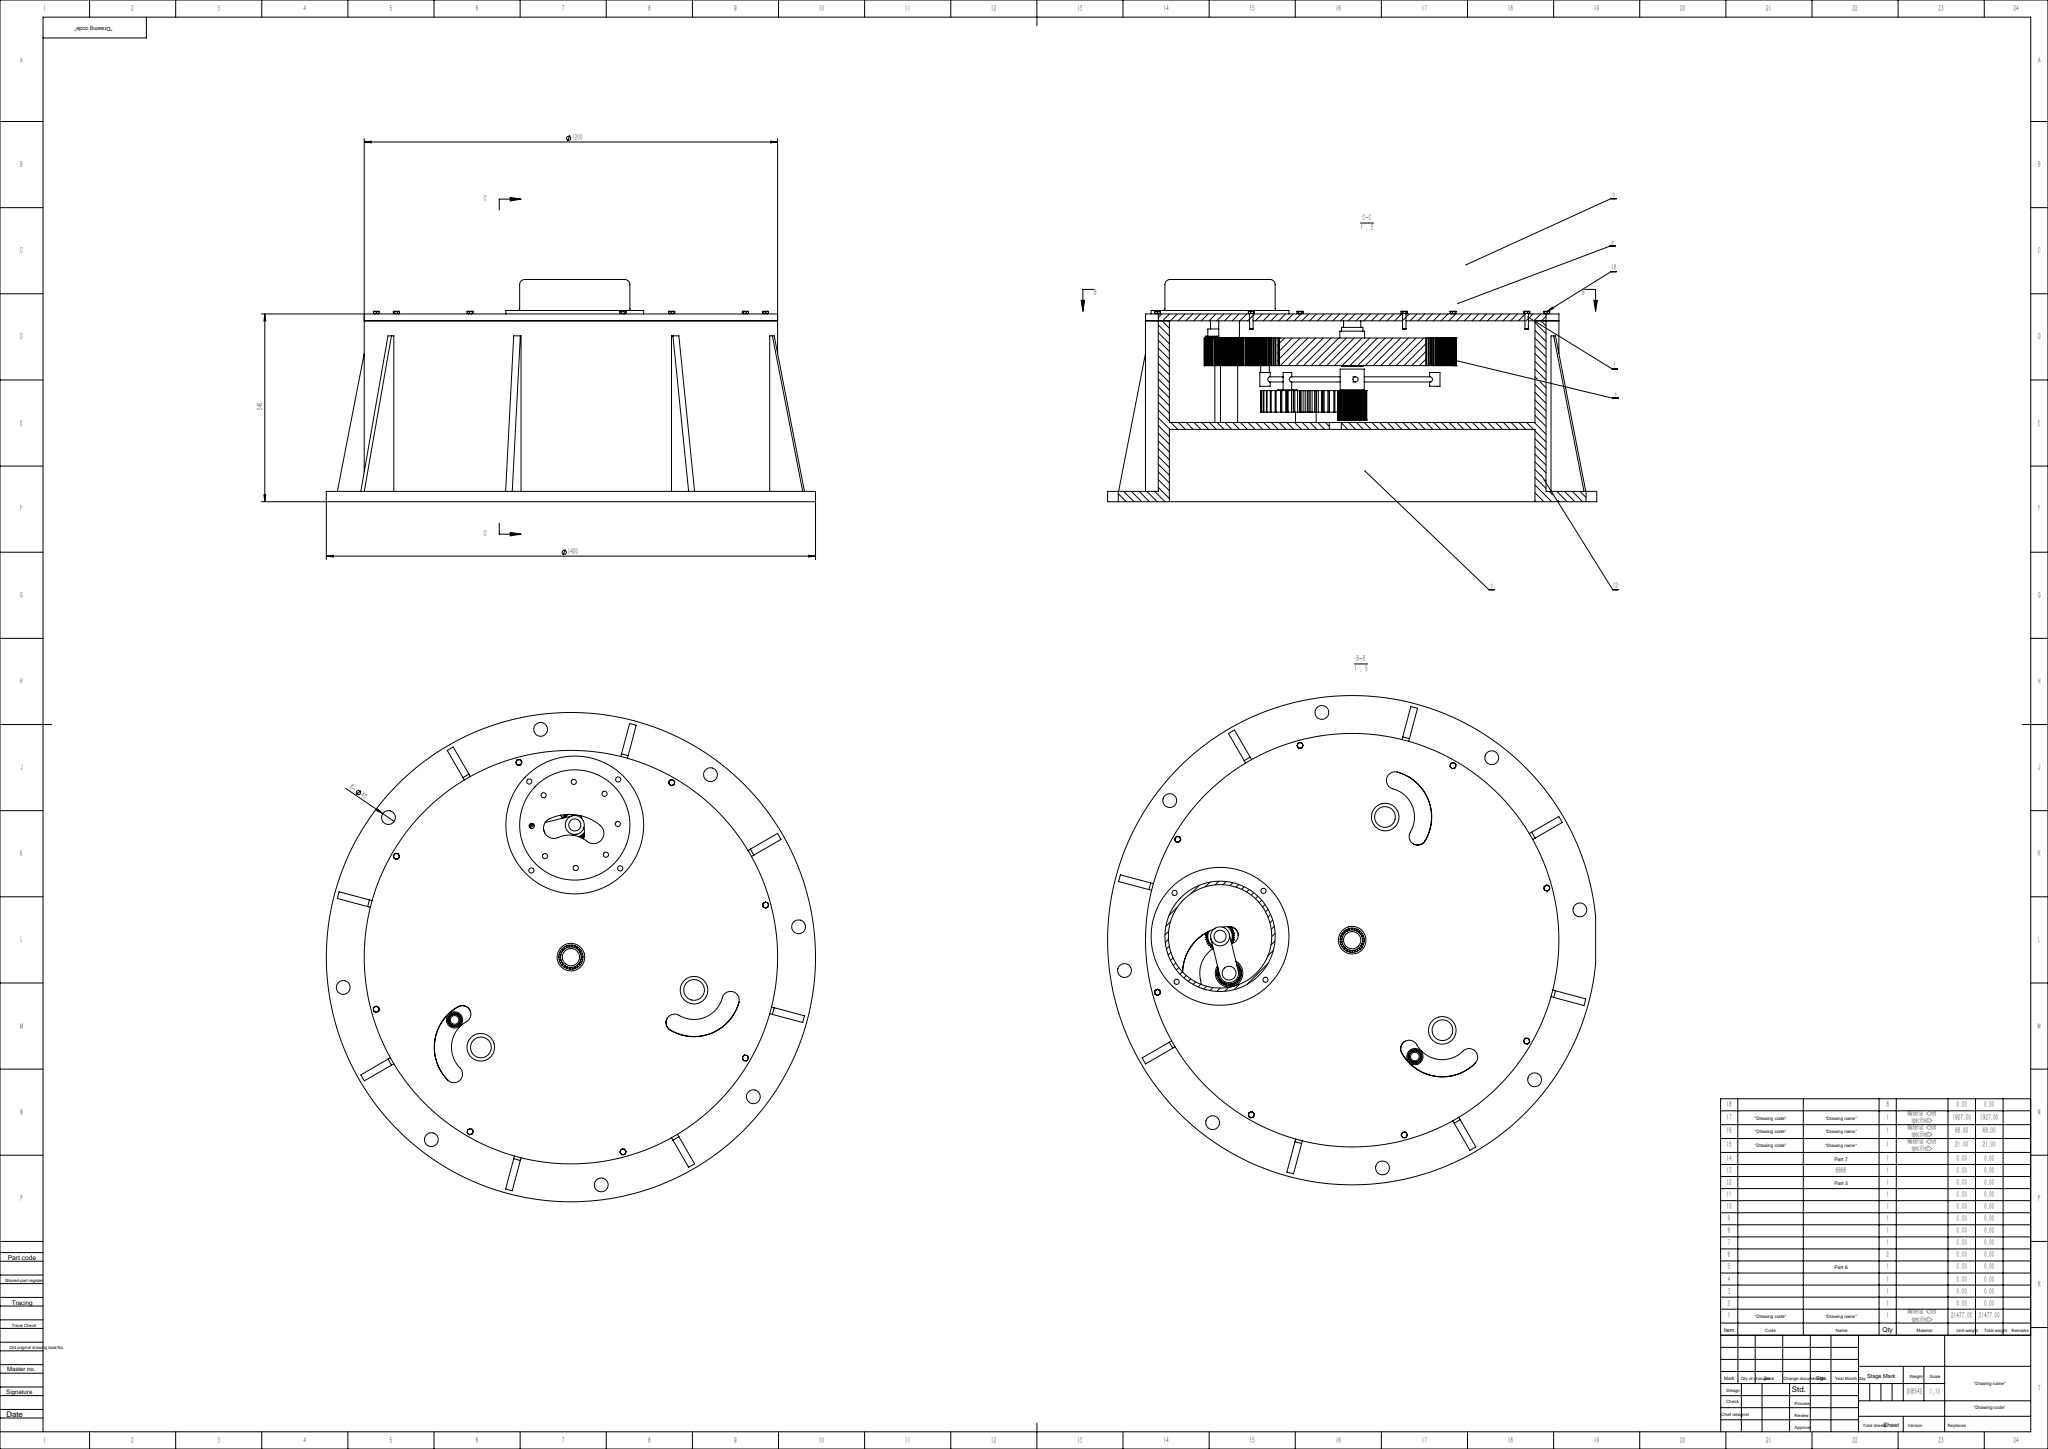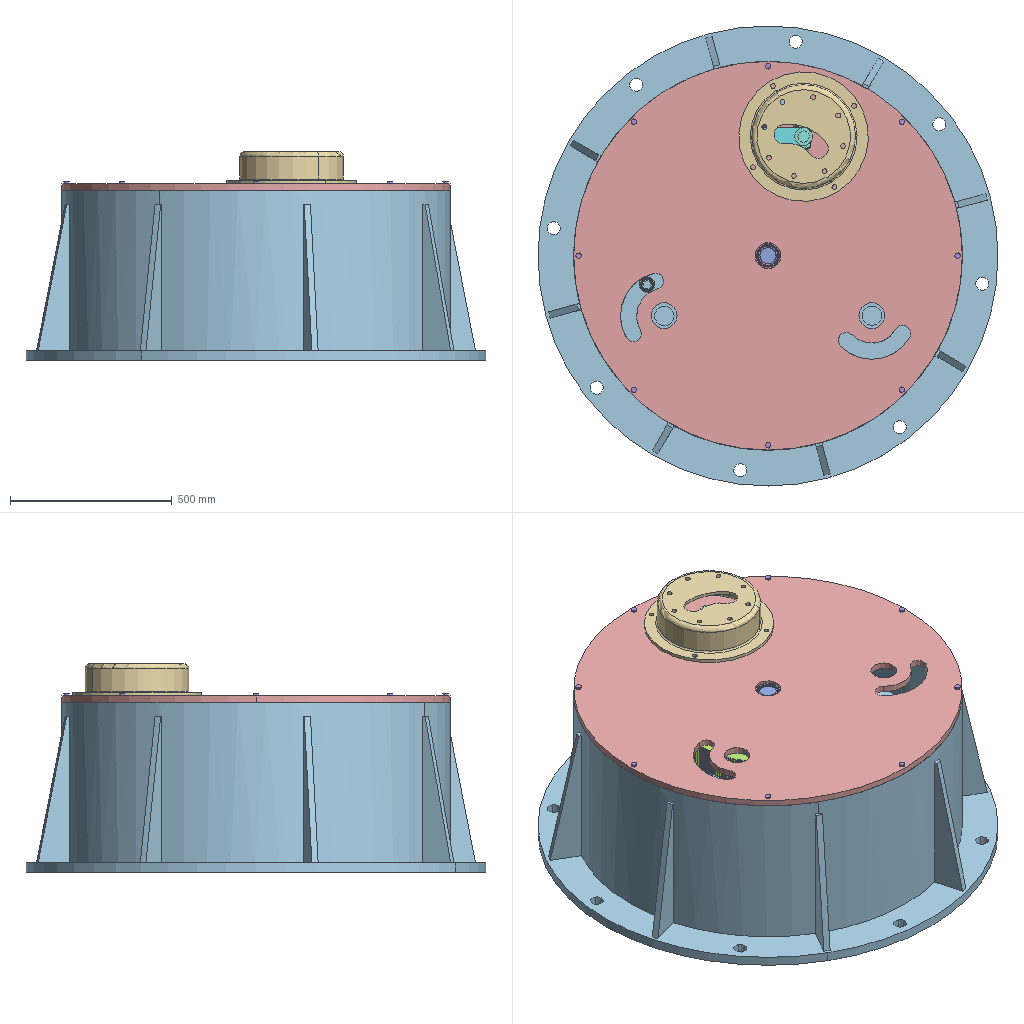Assembly | SolidWorks | 15 different items | 26 placed | box 1420 x 1420 x 645 mm
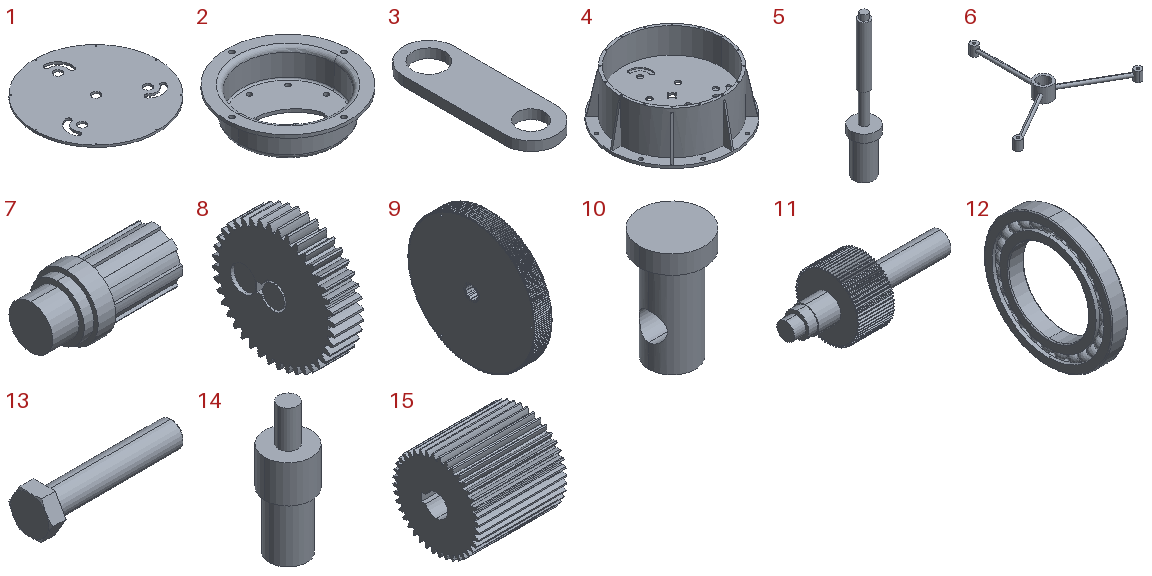Parts list (item | quantity | size | volume | features):
1 | x1 | 1200 x 1200 x 20 mm | 21477450 mm3 | features Extrusion 1
2 | x1 | 400 x 400 x 100 mm | 1926675 mm3 | features Fillet 2, ICE 2, Extrusion 1
3 | x1 | 55 x 165 x 10 mm | 67569 mm3 | features Extrusion 1
4 | x1 | 1420 x 1420 x 525 mm | 94468216 mm3 | features ICE 7, CirPattern 2, Cut 1, Extrusion 1
5 | x1 | 71 x 71 x 386.35 mm | 379556 mm3 | features ICE 4, Extrusion 1
6 | x1 | 523.634 x 457.5 x 60 mm | 315175 mm3 | features ICE 2, CirPattern 1, Extrusion 1
7 | x1 | 143 x 72 x 72 mm | 395287 mm3 | features ICE 2, CirPattern 1, Revolution 1
8 | x1 | 107.5 x 261.97 x 261.97 mm | 3068184 mm3 | features ICE 4, RefAxis 2, BaseBody 1, Chamfer 1, MoveFace 1, Revolution 1, Scale 1
9 | x1 | 80 x 604.968 x 604.968 mm | 22281815 mm3 | features Punch 2, BaseBody 1, CirPattern 1, HoleWzd 1, ICE 1
10 | x1 | 35 x 35 x 60 mm | 29956 mm3 | features ICE 2, Chamfer 1, Extrusion 1
11 | x1 | 350 x 143.909 x 144 mm | 1783229 mm3 | features ICE 4, Boss 3, Cut 3, CirPattern 2, Fillet 2, Revolution 1
12 | x4 | 10 x 80 x 80 mm | 24148 mm3 | features Revolution 3, CirPattern 1, Fillet 1
13 | x8 | 67.5 x 20.785 x 18 mm | 8849 mm3 | features RevCut 3, Boss 1, Chamfer 1, Extrusion 1, Fillet 1, LPattern 1
14 | x1 | 25 x 25 x 70 mm | 20813 mm3 | features ICE 2, Extrusion 1
15 | x2 | 85 x 83.831 x 83.831 mm | 385838 mm3 | features BaseBody 1
Mates (type | each side: item.copy, entity, surface, feature):
Concentric | 1.1 face cylinder Boss-Extrude1 | 7.1 face cylinder Revolve1
Concentric | 7.1 face cylinder Revolve1 | 9.1 face cylinder Input1
Coincident | 7.1 face plane Revolve1 | 9.1 face plane Input1
Coincident | 9.1 face plane Input1 | 11.1 face plane Base-Revolve
Concentric | 1.1 face cylinder Boss-Extrude1 | 11.1 face cylinder TeethCuts
DistanceDim | 9.1 face plane Input1 | 1.1 face plane Boss-Extrude1
Concentric | 5.1 face cylinder Boss-Extrude3 | 15.1 face cylinder Input1
Coincident | 5.1 face plane Boss-Extrude2 | 15.1 face plane Input1
Coincident | 11.1 face plane Base-Revolve | 15.1 face plane Input1
DistanceDim | 5.1 face cylinder Boss-Extrude3 | 11.1 face cylinder Bore
Coincident | 1.1 edge | 12.1 face cylinder Revolve3
Coincident | 1.1 face plane Boss-Extrude1 | 12.1 face plane Revolve3
Coincident | 8.1 face plane Cut-Extrude2 | 10.1 face plane Boss-Extrude1
Concentric | 8.1 face cylinder Cut-Extrude2 | 10.1 face cylinder Boss-Extrude1
Coincident | 8.1 face plane Cut-Extrude2 | 12.2 face plane Revolve2
Concentric | 10.1 face cylinder Boss-Extrude1 | 12.2 face cylinder Revolve3
Coincident | 8.1 face plane Revolve1 | 4.1 face plane Boss-Extrude1
Concentric | 1.1 face cylinder Boss-Extrude1 | 6.1 face cylinder Boss-Extrude1
Concentric | 10.1 face cylinder Cut-Extrude1 | 6.1 face cylinder CirPattern3
Concentric | 9.1 face cylinder CirPattern2 | 6.1 face cylinder CirPattern3
Concentric | 6.1 face cylinder CirPattern3 | 14.1 face cylinder Boss-Extrude3
Coincident | 9.1 face plane Input1 | 14.1 face plane Boss-Extrude2
Coincident | 4.1 face plane Boss-Extrude1 | 12.3 face plane Revolve2
Concentric | 1.1 face cylinder Boss-Extrude1 | 12.4 face cylinder Revolve3
Coincident | 7.1 face plane Boss-Extrude2 | 12.4 face plane Revolve3
Concentric | 11.1 face cylinder Boss-Extrude5 | 3.1 face cylinder Boss-Extrude1
Tangent | 5.1 face cylinder Boss-Extrude1 | 3.1 face plane Boss-Extrude1
Concentric | 8.1 face cylinder Revolve1 | 4.1 edge
Concentric | 1.1 face cylinder Boss-Extrude1 | 13.1 face cylinder BaseBody
Coincident | 1.1 face plane Boss-Extrude1 | 2.1 face plane Boss-Extrude3